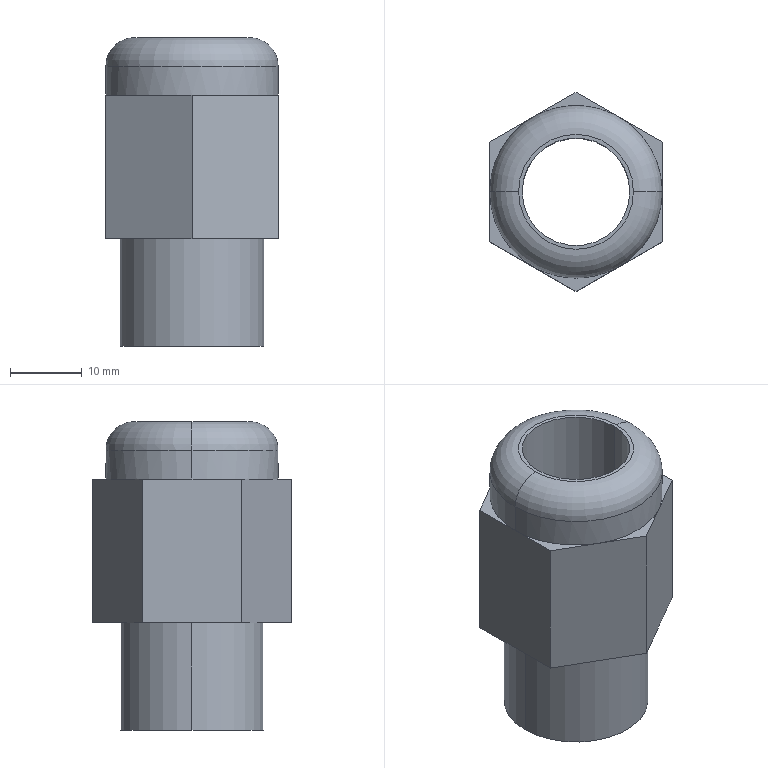Part | SolidWorks | features ICE 2, Extrusion 1, Fillet 1 | 1 solid | 23 faces | box 24 x 27.713 x 43 mm | volume 10470 mm3 | plane 15 | cylinder 6 | torus 2 | commonest cylinder face diameters 15 x2 20 x2 24 x2
STEP:
#1=CARTESIAN_POINT('',(-10.,0.,-15.));
#2=VERTEX_POINT('',#1);
#3=CARTESIAN_POINT('',(10.,0.,-15.));
#4=VERTEX_POINT('',#3);
#5=CARTESIAN_POINT('',(0.,0.,-15.));
#6=DIRECTION('',(0.,0.,-1.));
#7=DIRECTION('',(-1.,0.,0.));
#8=AXIS2_PLACEMENT_3D('',#5,#6,#7);
#9=CIRCLE('',#8,10.);
#10=EDGE_CURVE('',#2,#4,#9,.T.);
#11=ORIENTED_EDGE('',*,*,#10,.F.);
#12=CARTESIAN_POINT('',(-10.,0.,0.));
#13=VERTEX_POINT('',#12);
#14=CARTESIAN_POINT('',(-10.,0.,-15.));
#15=DIRECTION('',(0.,0.,1.));
#16=VECTOR('',#15,1000.);
#17=LINE('',#14,#16);
#18=EDGE_CURVE('',#2,#13,#17,.T.);
#19=ORIENTED_EDGE('',*,*,#18,.T.);
#20=CARTESIAN_POINT('',(10.,0.,0.));
#21=VERTEX_POINT('',#20);
#22=CARTESIAN_POINT('',(0.,0.,0.));
#23=DIRECTION('',(0.,0.,-1.));
#24=DIRECTION('',(1.,0.,0.));
#25=AXIS2_PLACEMENT_3D('',#22,#23,#24);
#26=CIRCLE('',#25,10.);
#27=EDGE_CURVE('',#13,#21,#26,.T.);
#28=ORIENTED_EDGE('',*,*,#27,.T.);
#29=CARTESIAN_POINT('',(10.,0.,-15.));
#30=DIRECTION('',(0.,0.,1.));
#31=VECTOR('',#30,1000.);
#32=LINE('',#29,#31);
#33=EDGE_CURVE('',#4,#21,#32,.T.);
#34=ORIENTED_EDGE('',*,*,#33,.F.);
#35=EDGE_LOOP('',(#11,#19,#28,#34));
#36=FACE_OUTER_BOUND('',#35,.T.);
#37=CARTESIAN_POINT('',(0.,0.,-15.));
#38=DIRECTION('',(0.,0.,1.));
#39=DIRECTION('',(1.,0.,0.));
#40=AXIS2_PLACEMENT_3D('',#37,#38,#39);
#41=CYLINDRICAL_SURFACE('',#40,10.);
#42=ADVANCED_FACE('',(#36),#41,.T.);
#43=CARTESIAN_POINT('',(-12.,0.,24.));
#44=VERTEX_POINT('',#43);
#45=CARTESIAN_POINT('',(12.,0.,24.));
#46=VERTEX_POINT('',#45);
#47=CARTESIAN_POINT('',(0.,0.,24.));
#48=DIRECTION('',(0.,0.,-1.));
#49=DIRECTION('',(1.,0.,0.));
#50=AXIS2_PLACEMENT_3D('',#47,#48,#49);
#51=CIRCLE('',#50,12.);
#52=EDGE_CURVE('',#44,#46,#51,.T.);
#53=ORIENTED_EDGE('',*,*,#52,.F.);
#54=CARTESIAN_POINT('',(-8.,0.,28.));
#55=VERTEX_POINT('',#54);
#56=CARTESIAN_POINT('',(-8.,0.,24.));
#57=DIRECTION('',(0.,1.,0.));
#58=DIRECTION('',(-1.,0.,0.));
#59=AXIS2_PLACEMENT_3D('',#56,#57,#58);
#60=CIRCLE('',#59,4.);
#61=EDGE_CURVE('',#44,#55,#60,.T.);
#62=ORIENTED_EDGE('',*,*,#61,.T.);
#63=CARTESIAN_POINT('',(8.,0.,28.));
#64=VERTEX_POINT('',#63);
#65=CARTESIAN_POINT('',(0.,0.,28.));
#66=DIRECTION('',(0.,0.,1.));
#67=DIRECTION('',(1.,0.,0.));
#68=AXIS2_PLACEMENT_3D('',#65,#66,#67);
#69=CIRCLE('',#68,8.);
#70=EDGE_CURVE('',#64,#55,#69,.T.);
#71=ORIENTED_EDGE('',*,*,#70,.F.);
#72=CARTESIAN_POINT('',(8.,0.,24.));
#73=DIRECTION('',(0.,-1.,0.));
#74=DIRECTION('',(0.,0.,-1.));
#75=AXIS2_PLACEMENT_3D('',#72,#73,#74);
#76=CIRCLE('',#75,4.);
#77=EDGE_CURVE('',#46,#64,#76,.T.);
#78=ORIENTED_EDGE('',*,*,#77,.F.);
#79=EDGE_LOOP('',(#53,#62,#71,#78));
#80=FACE_OUTER_BOUND('',#79,.T.);
#81=CARTESIAN_POINT('',(0.,0.,24.));
#82=DIRECTION('',(0.,0.,1.));
#83=DIRECTION('',(1.,0.,0.));
#84=AXIS2_PLACEMENT_3D('',#81,#82,#83);
#85=TOROIDAL_SURFACE('',#84,8.,4.);
#86=ADVANCED_FACE('',(#80),#85,.T.);
#87=ORIENTED_EDGE('',*,*,#52,.T.);
#88=CARTESIAN_POINT('',(12.,0.,20.));
#89=VERTEX_POINT('',#88);
#90=CARTESIAN_POINT('',(12.,0.,28.));
#91=DIRECTION('',(0.,0.,-1.));
#92=VECTOR('',#91,1000.);
#93=LINE('',#90,#92);
#94=EDGE_CURVE('',#46,#89,#93,.T.);
#95=ORIENTED_EDGE('',*,*,#94,.T.);
#96=CARTESIAN_POINT('',(6.,10.392,20.));
#97=VERTEX_POINT('',#96);
#98=CARTESIAN_POINT('',(0.,0.,20.));
#99=DIRECTION('',(0.,0.,1.));
#100=DIRECTION('',(1.,0.,0.));
#101=AXIS2_PLACEMENT_3D('',#98,#99,#100);
#102=CIRCLE('',#101,12.);
#103=EDGE_CURVE('',#89,#97,#102,.T.);
#104=ORIENTED_EDGE('',*,*,#103,.T.);
#105=CARTESIAN_POINT('',(-6.,10.392,20.));
#106=VERTEX_POINT('',#105);
#107=CARTESIAN_POINT('',(0.,0.,20.));
#108=DIRECTION('',(0.,0.,1.));
#109=DIRECTION('',(1.,0.,0.));
#110=AXIS2_PLACEMENT_3D('',#107,#108,#109);
#111=CIRCLE('',#110,12.);
#112=EDGE_CURVE('',#97,#106,#111,.T.);
#113=ORIENTED_EDGE('',*,*,#112,.T.);
#114=CARTESIAN_POINT('',(-12.,0.,20.));
#115=VERTEX_POINT('',#114);
#116=CARTESIAN_POINT('',(0.,0.,20.));
#117=DIRECTION('',(0.,0.,1.));
#118=DIRECTION('',(1.,0.,0.));
#119=AXIS2_PLACEMENT_3D('',#116,#117,#118);
#120=CIRCLE('',#119,12.);
#121=EDGE_CURVE('',#106,#115,#120,.T.);
#122=ORIENTED_EDGE('',*,*,#121,.T.);
#123=CARTESIAN_POINT('',(-12.,0.,28.));
#124=DIRECTION('',(0.,0.,-1.));
#125=VECTOR('',#124,1000.);
#126=LINE('',#123,#125);
#127=EDGE_CURVE('',#44,#115,#126,.T.);
#128=ORIENTED_EDGE('',*,*,#127,.F.);
#129=EDGE_LOOP('',(#87,#95,#104,#113,#122,#128));
#130=FACE_OUTER_BOUND('',#129,.T.);
#131=CARTESIAN_POINT('',(0.,0.,28.));
#132=DIRECTION('',(0.,0.,-1.));
#133=DIRECTION('',(-1.,0.,0.));
#134=AXIS2_PLACEMENT_3D('',#131,#132,#133);
#135=CYLINDRICAL_SURFACE('',#134,12.);
#136=ADVANCED_FACE('',(#130),#135,.T.);
#137=CARTESIAN_POINT('',(-7.5,0.,28.));
#138=VERTEX_POINT('',#137);
#139=CARTESIAN_POINT('',(7.5,0.,28.));
#140=VERTEX_POINT('',#139);
#141=CARTESIAN_POINT('',(0.,0.,28.));
#142=DIRECTION('',(0.,0.,1.));
#143=DIRECTION('',(1.,0.,0.));
#144=AXIS2_PLACEMENT_3D('',#141,#142,#143);
#145=CIRCLE('',#144,7.5);
#146=EDGE_CURVE('',#138,#140,#145,.T.);
#147=ORIENTED_EDGE('',*,*,#146,.T.);
#148=CARTESIAN_POINT('',(7.5,0.,-15.));
#149=VERTEX_POINT('',#148);
#150=CARTESIAN_POINT('',(7.5,0.,20.));
#151=DIRECTION('',(0.,0.,-1.));
#152=VECTOR('',#151,1000.);
#153=LINE('',#150,#152);
#154=EDGE_CURVE('',#140,#149,#153,.T.);
#155=ORIENTED_EDGE('',*,*,#154,.T.);
#156=CARTESIAN_POINT('',(-7.5,0.,-15.));
#157=VERTEX_POINT('',#156);
#158=CARTESIAN_POINT('',(0.,0.,-15.));
#159=DIRECTION('',(0.,0.,-1.));
#160=DIRECTION('',(-1.,0.,0.));
#161=AXIS2_PLACEMENT_3D('',#158,#159,#160);
#162=CIRCLE('',#161,7.5);
#163=EDGE_CURVE('',#149,#157,#162,.T.);
#164=ORIENTED_EDGE('',*,*,#163,.T.);
#165=CARTESIAN_POINT('',(-7.5,0.,20.));
#166=DIRECTION('',(0.,0.,-1.));
#167=VECTOR('',#166,1000.);
#168=LINE('',#165,#167);
#169=EDGE_CURVE('',#138,#157,#168,.T.);
#170=ORIENTED_EDGE('',*,*,#169,.F.);
#171=EDGE_LOOP('',(#147,#155,#164,#170));
#172=FACE_OUTER_BOUND('',#171,.T.);
#173=CARTESIAN_POINT('',(0.,0.,20.));
#174=DIRECTION('',(0.,0.,-1.));
#175=DIRECTION('',(-1.,0.,0.));
#176=AXIS2_PLACEMENT_3D('',#173,#174,#175);
#177=CYLINDRICAL_SURFACE('',#176,7.5);
#178=ADVANCED_FACE('',(#172),#177,.F.);
#179=CARTESIAN_POINT('',(12.,6.928,0.));
#180=VERTEX_POINT('',#179);
#181=CARTESIAN_POINT('',(0.,13.856,0.));
#182=VERTEX_POINT('',#181);
#183=CARTESIAN_POINT('',(12.,6.928,0.));
#184=DIRECTION('',(-0.866,0.5,0.));
#185=VECTOR('',#184,1000.);
#186=LINE('',#183,#185);
#187=EDGE_CURVE('',#180,#182,#186,.T.);
#188=ORIENTED_EDGE('',*,*,#187,.F.);
#189=CARTESIAN_POINT('',(12.,-6.928,0.));
#190=VERTEX_POINT('',#189);
#191=CARTESIAN_POINT('',(12.,-6.928,0.));
#192=DIRECTION('',(0.,1.,0.));
#193=VECTOR('',#192,1000.);
#194=LINE('',#191,#193);
#195=EDGE_CURVE('',#190,#180,#194,.T.);
#196=ORIENTED_EDGE('',*,*,#195,.F.);
#197=CARTESIAN_POINT('',(0.,-13.856,0.));
#198=VERTEX_POINT('',#197);
#199=CARTESIAN_POINT('',(0.,-13.856,0.));
#200=DIRECTION('',(0.866,0.5,0.));
#201=VECTOR('',#200,1000.);
#202=LINE('',#199,#201);
#203=EDGE_CURVE('',#198,#190,#202,.T.);
#204=ORIENTED_EDGE('',*,*,#203,.F.);
#205=CARTESIAN_POINT('',(-12.,-6.928,0.));
#206=VERTEX_POINT('',#205);
#207=CARTESIAN_POINT('',(-12.,-6.928,0.));
#208=DIRECTION('',(0.866,-0.5,0.));
#209=VECTOR('',#208,1000.);
#210=LINE('',#207,#209);
#211=EDGE_CURVE('',#206,#198,#210,.T.);
#212=ORIENTED_EDGE('',*,*,#211,.F.);
#213=CARTESIAN_POINT('',(-12.,6.928,0.));
#214=VERTEX_POINT('',#213);
#215=CARTESIAN_POINT('',(-12.,6.928,0.));
#216=DIRECTION('',(0.,-1.,0.));
#217=VECTOR('',#216,1000.);
#218=LINE('',#215,#217);
#219=EDGE_CURVE('',#214,#206,#218,.T.);
#220=ORIENTED_EDGE('',*,*,#219,.F.);
#221=CARTESIAN_POINT('',(0.,13.856,0.));
#222=DIRECTION('',(-0.866,-0.5,0.));
#223=VECTOR('',#222,1000.);
#224=LINE('',#221,#223);
#225=EDGE_CURVE('',#182,#214,#224,.T.);
#226=ORIENTED_EDGE('',*,*,#225,.F.);
#227=EDGE_LOOP('',(#188,#196,#204,#212,#220,#226));
#228=FACE_OUTER_BOUND('',#227,.T.);
#229=CARTESIAN_POINT('',(0.,0.,0.));
#230=DIRECTION('',(0.,0.,-1.));
#231=DIRECTION('',(1.,0.,0.));
#232=AXIS2_PLACEMENT_3D('',#229,#230,#231);
#233=CIRCLE('',#232,10.);
#234=EDGE_CURVE('',#21,#13,#233,.T.);
#235=ORIENTED_EDGE('',*,*,#234,.F.);
#236=ORIENTED_EDGE('',*,*,#27,.F.);
#237=EDGE_LOOP('',(#235,#236));
#238=FACE_BOUND('',#237,.T.);
#239=CARTESIAN_POINT('',(0.,0.,0.));
#240=DIRECTION('',(0.,0.,1.));
#241=DIRECTION('',(1.,0.,0.));
#242=AXIS2_PLACEMENT_3D('',#239,#240,#241);
#243=PLANE('',#242);
#244=ADVANCED_FACE('',(#228,#238),#243,.F.);
#245=ORIENTED_EDGE('',*,*,#103,.F.);
#246=CARTESIAN_POINT('',(12.,6.928,20.));
#247=VERTEX_POINT('',#246);
#248=CARTESIAN_POINT('',(12.,-6.928,20.));
#249=DIRECTION('',(0.,1.,0.));
#250=VECTOR('',#249,1000.);
#251=LINE('',#248,#250);
#252=EDGE_CURVE('',#89,#247,#251,.T.);
#253=ORIENTED_EDGE('',*,*,#252,.T.);
#254=CARTESIAN_POINT('',(12.,6.928,20.));
#255=DIRECTION('',(-0.866,0.5,0.));
#256=VECTOR('',#255,1000.);
#257=LINE('',#254,#256);
#258=EDGE_CURVE('',#247,#97,#257,.T.);
#259=ORIENTED_EDGE('',*,*,#258,.T.);
#260=EDGE_LOOP('',(#245,#253,#259));
#261=FACE_OUTER_BOUND('',#260,.T.);
#262=CARTESIAN_POINT('',(0.,0.,20.));
#263=DIRECTION('',(0.,0.,1.));
#264=DIRECTION('',(1.,0.,0.));
#265=AXIS2_PLACEMENT_3D('',#262,#263,#264);
#266=PLANE('',#265);
#267=ADVANCED_FACE('',(#261),#266,.T.);
#268=ORIENTED_EDGE('',*,*,#112,.F.);
#269=CARTESIAN_POINT('',(0.,13.856,20.));
#270=VERTEX_POINT('',#269);
#271=CARTESIAN_POINT('',(12.,6.928,20.));
#272=DIRECTION('',(-0.866,0.5,0.));
#273=VECTOR('',#272,1000.);
#274=LINE('',#271,#273);
#275=EDGE_CURVE('',#97,#270,#274,.T.);
#276=ORIENTED_EDGE('',*,*,#275,.T.);
#277=CARTESIAN_POINT('',(0.,13.856,20.));
#278=DIRECTION('',(-0.866,-0.5,0.));
#279=VECTOR('',#278,1000.);
#280=LINE('',#277,#279);
#281=EDGE_CURVE('',#270,#106,#280,.T.);
#282=ORIENTED_EDGE('',*,*,#281,.T.);
#283=EDGE_LOOP('',(#268,#276,#282));
#284=FACE_OUTER_BOUND('',#283,.T.);
#285=CARTESIAN_POINT('',(0.,0.,20.));
#286=DIRECTION('',(0.,0.,1.));
#287=DIRECTION('',(1.,0.,0.));
#288=AXIS2_PLACEMENT_3D('',#285,#286,#287);
#289=PLANE('',#288);
#290=ADVANCED_FACE('',(#284),#289,.T.);
#291=ORIENTED_EDGE('',*,*,#121,.F.);
#292=CARTESIAN_POINT('',(-12.,6.928,20.));
#293=VERTEX_POINT('',#292);
#294=CARTESIAN_POINT('',(0.,13.856,20.));
#295=DIRECTION('',(-0.866,-0.5,0.));
#296=VECTOR('',#295,1000.);
#297=LINE('',#294,#296);
#298=EDGE_CURVE('',#106,#293,#297,.T.);
#299=ORIENTED_EDGE('',*,*,#298,.T.);
#300=CARTESIAN_POINT('',(-12.,6.928,20.));
#301=DIRECTION('',(0.,-1.,0.));
#302=VECTOR('',#301,1000.);
#303=LINE('',#300,#302);
#304=EDGE_CURVE('',#293,#115,#303,.T.);
#305=ORIENTED_EDGE('',*,*,#304,.T.);
#306=EDGE_LOOP('',(#291,#299,#305));
#307=FACE_OUTER_BOUND('',#306,.T.);
#308=CARTESIAN_POINT('',(0.,0.,20.));
#309=DIRECTION('',(0.,0.,1.));
#310=DIRECTION('',(1.,0.,0.));
#311=AXIS2_PLACEMENT_3D('',#308,#309,#310);
#312=PLANE('',#311);
#313=ADVANCED_FACE('',(#307),#312,.T.);
#314=CARTESIAN_POINT('',(-6.,-10.392,20.));
#315=VERTEX_POINT('',#314);
#316=CARTESIAN_POINT('',(0.,0.,20.));
#317=DIRECTION('',(0.,0.,1.));
#318=DIRECTION('',(1.,0.,0.));
#319=AXIS2_PLACEMENT_3D('',#316,#317,#318);
#320=CIRCLE('',#319,12.);
#321=EDGE_CURVE('',#115,#315,#320,.T.);
#322=ORIENTED_EDGE('',*,*,#321,.F.);
#323=CARTESIAN_POINT('',(-12.,-6.928,20.));
#324=VERTEX_POINT('',#323);
#325=CARTESIAN_POINT('',(-12.,6.928,20.));
#326=DIRECTION('',(0.,-1.,0.));
#327=VECTOR('',#326,1000.);
#328=LINE('',#325,#327);
#329=EDGE_CURVE('',#115,#324,#328,.T.);
#330=ORIENTED_EDGE('',*,*,#329,.T.);
#331=CARTESIAN_POINT('',(-12.,-6.928,20.));
#332=DIRECTION('',(0.866,-0.5,0.));
#333=VECTOR('',#332,1000.);
#334=LINE('',#331,#333);
#335=EDGE_CURVE('',#324,#315,#334,.T.);
#336=ORIENTED_EDGE('',*,*,#335,.T.);
#337=EDGE_LOOP('',(#322,#330,#336));
#338=FACE_OUTER_BOUND('',#337,.T.);
#339=CARTESIAN_POINT('',(0.,0.,20.));
#340=DIRECTION('',(0.,0.,1.));
#341=DIRECTION('',(1.,0.,0.));
#342=AXIS2_PLACEMENT_3D('',#339,#340,#341);
#343=PLANE('',#342);
#344=ADVANCED_FACE('',(#338),#343,.T.);
#345=CARTESIAN_POINT('',(6.,-10.392,20.));
#346=VERTEX_POINT('',#345);
#347=CARTESIAN_POINT('',(0.,0.,20.));
#348=DIRECTION('',(0.,0.,1.));
#349=DIRECTION('',(1.,0.,0.));
#350=AXIS2_PLACEMENT_3D('',#347,#348,#349);
#351=CIRCLE('',#350,12.);
#352=EDGE_CURVE('',#315,#346,#351,.T.);
#353=ORIENTED_EDGE('',*,*,#352,.F.);
#354=CARTESIAN_POINT('',(0.,-13.856,20.));
#355=VERTEX_POINT('',#354);
#356=CARTESIAN_POINT('',(-12.,-6.928,20.));
#357=DIRECTION('',(0.866,-0.5,0.));
#358=VECTOR('',#357,1000.);
#359=LINE('',#356,#358);
#360=EDGE_CURVE('',#315,#355,#359,.T.);
#361=ORIENTED_EDGE('',*,*,#360,.T.);
#362=CARTESIAN_POINT('',(0.,-13.856,20.));
#363=DIRECTION('',(0.866,0.5,0.));
#364=VECTOR('',#363,1000.);
#365=LINE('',#362,#364);
#366=EDGE_CURVE('',#355,#346,#365,.T.);
#367=ORIENTED_EDGE('',*,*,#366,.T.);
#368=EDGE_LOOP('',(#353,#361,#367));
#369=FACE_OUTER_BOUND('',#368,.T.);
#370=CARTESIAN_POINT('',(0.,0.,20.));
#371=DIRECTION('',(0.,0.,1.));
#372=DIRECTION('',(1.,0.,0.));
#373=AXIS2_PLACEMENT_3D('',#370,#371,#372);
#374=PLANE('',#373);
#375=ADVANCED_FACE('',(#369),#374,.T.);
#376=CARTESIAN_POINT('',(0.,0.,20.));
#377=DIRECTION('',(0.,0.,1.));
#378=DIRECTION('',(1.,0.,0.));
#379=AXIS2_PLACEMENT_3D('',#376,#377,#378);
#380=CIRCLE('',#379,12.);
#381=EDGE_CURVE('',#346,#89,#380,.T.);
#382=ORIENTED_EDGE('',*,*,#381,.F.);
#383=CARTESIAN_POINT('',(12.,-6.928,20.));
#384=VERTEX_POINT('',#383);
#385=CARTESIAN_POINT('',(0.,-13.856,20.));
#386=DIRECTION('',(0.866,0.5,0.));
#387=VECTOR('',#386,1000.);
#388=LINE('',#385,#387);
#389=EDGE_CURVE('',#346,#384,#388,.T.);
#390=ORIENTED_EDGE('',*,*,#389,.T.);
#391=CARTESIAN_POINT('',(12.,-6.928,20.));
#392=DIRECTION('',(0.,1.,0.));
#393=VECTOR('',#392,1000.);
#394=LINE('',#391,#393);
#395=EDGE_CURVE('',#384,#89,#394,.T.);
#396=ORIENTED_EDGE('',*,*,#395,.T.);
#397=EDGE_LOOP('',(#382,#390,#396));
#398=FACE_OUTER_BOUND('',#397,.T.);
#399=CARTESIAN_POINT('',(0.,0.,20.));
#400=DIRECTION('',(0.,0.,1.));
#401=DIRECTION('',(1.,0.,0.));
#402=AXIS2_PLACEMENT_3D('',#399,#400,#401);
#403=PLANE('',#402);
#404=ADVANCED_FACE('',(#398),#403,.T.);
#405=ORIENTED_EDGE('',*,*,#187,.T.);
#406=CARTESIAN_POINT('',(0.,13.856,20.));
#407=DIRECTION('',(0.,0.,-1.));
#408=VECTOR('',#407,1000.);
#409=LINE('',#406,#408);
#410=EDGE_CURVE('',#270,#182,#409,.T.);
#411=ORIENTED_EDGE('',*,*,#410,.F.);
#412=ORIENTED_EDGE('',*,*,#275,.F.);
#413=ORIENTED_EDGE('',*,*,#258,.F.);
#414=CARTESIAN_POINT('',(12.,6.928,20.));
#415=DIRECTION('',(0.,0.,-1.));
#416=VECTOR('',#415,1000.);
#417=LINE('',#414,#416);
#418=EDGE_CURVE('',#247,#180,#417,.T.);
#419=ORIENTED_EDGE('',*,*,#418,.T.);
#420=EDGE_LOOP('',(#405,#411,#412,#413,#419));
#421=FACE_OUTER_BOUND('',#420,.T.);
#422=CARTESIAN_POINT('',(12.,6.928,20.));
#423=DIRECTION('',(-0.5,-0.866,0.));
#424=DIRECTION('',(0.866,-0.5,0.));
#425=AXIS2_PLACEMENT_3D('',#422,#423,#424);
#426=PLANE('',#425);
#427=ADVANCED_FACE('',(#421),#426,.F.);
#428=ORIENTED_EDGE('',*,*,#225,.T.);
#429=CARTESIAN_POINT('',(-12.,6.928,20.));
#430=DIRECTION('',(0.,0.,-1.));
#431=VECTOR('',#430,1000.);
#432=LINE('',#429,#431);
#433=EDGE_CURVE('',#293,#214,#432,.T.);
#434=ORIENTED_EDGE('',*,*,#433,.F.);
#435=ORIENTED_EDGE('',*,*,#298,.F.);
#436=ORIENTED_EDGE('',*,*,#281,.F.);
#437=ORIENTED_EDGE('',*,*,#410,.T.);
#438=EDGE_LOOP('',(#428,#434,#435,#436,#437));
#439=FACE_OUTER_BOUND('',#438,.T.);
#440=CARTESIAN_POINT('',(0.,13.856,20.));
#441=DIRECTION('',(0.5,-0.866,0.));
#442=DIRECTION('',(0.866,0.5,0.));
#443=AXIS2_PLACEMENT_3D('',#440,#441,#442);
#444=PLANE('',#443);
#445=ADVANCED_FACE('',(#439),#444,.F.);
#446=ORIENTED_EDGE('',*,*,#219,.T.);
#447=CARTESIAN_POINT('',(-12.,-6.928,20.));
#448=DIRECTION('',(0.,0.,-1.));
#449=VECTOR('',#448,1000.);
#450=LINE('',#447,#449);
#451=EDGE_CURVE('',#324,#206,#450,.T.);
#452=ORIENTED_EDGE('',*,*,#451,.F.);
#453=ORIENTED_EDGE('',*,*,#329,.F.);
#454=ORIENTED_EDGE('',*,*,#304,.F.);
#455=ORIENTED_EDGE('',*,*,#433,.T.);
#456=EDGE_LOOP('',(#446,#452,#453,#454,#455));
#457=FACE_OUTER_BOUND('',#456,.T.);
#458=CARTESIAN_POINT('',(-12.,6.928,20.));
#459=DIRECTION('',(1.,0.,0.));
#460=DIRECTION('',(0.,1.,0.));
#461=AXIS2_PLACEMENT_3D('',#458,#459,#460);
#462=PLANE('',#461);
#463=ADVANCED_FACE('',(#457),#462,.F.);
#464=ORIENTED_EDGE('',*,*,#211,.T.);
#465=CARTESIAN_POINT('',(0.,-13.856,20.));
#466=DIRECTION('',(0.,0.,-1.));
#467=VECTOR('',#466,1000.);
#468=LINE('',#465,#467);
#469=EDGE_CURVE('',#355,#198,#468,.T.);
#470=ORIENTED_EDGE('',*,*,#469,.F.);
#471=ORIENTED_EDGE('',*,*,#360,.F.);
#472=ORIENTED_EDGE('',*,*,#335,.F.);
#473=ORIENTED_EDGE('',*,*,#451,.T.);
#474=EDGE_LOOP('',(#464,#470,#471,#472,#473));
#475=FACE_OUTER_BOUND('',#474,.T.);
#476=CARTESIAN_POINT('',(-12.,-6.928,20.));
#477=DIRECTION('',(0.5,0.866,0.));
#478=DIRECTION('',(-0.866,0.5,0.));
#479=AXIS2_PLACEMENT_3D('',#476,#477,#478);
#480=PLANE('',#479);
#481=ADVANCED_FACE('',(#475),#480,.F.);
#482=ORIENTED_EDGE('',*,*,#203,.T.);
#483=CARTESIAN_POINT('',(12.,-6.928,20.));
#484=DIRECTION('',(0.,0.,-1.));
#485=VECTOR('',#484,1000.);
#486=LINE('',#483,#485);
#487=EDGE_CURVE('',#384,#190,#486,.T.);
#488=ORIENTED_EDGE('',*,*,#487,.F.);
#489=ORIENTED_EDGE('',*,*,#389,.F.);
#490=ORIENTED_EDGE('',*,*,#366,.F.);
#491=ORIENTED_EDGE('',*,*,#469,.T.);
#492=EDGE_LOOP('',(#482,#488,#489,#490,#491));
#493=FACE_OUTER_BOUND('',#492,.T.);
#494=CARTESIAN_POINT('',(0.,-13.856,20.));
#495=DIRECTION('',(-0.5,0.866,0.));
#496=DIRECTION('',(-0.866,-0.5,0.));
#497=AXIS2_PLACEMENT_3D('',#494,#495,#496);
#498=PLANE('',#497);
#499=ADVANCED_FACE('',(#493),#498,.F.);
#500=ORIENTED_EDGE('',*,*,#195,.T.);
#501=ORIENTED_EDGE('',*,*,#418,.F.);
#502=ORIENTED_EDGE('',*,*,#252,.F.);
#503=ORIENTED_EDGE('',*,*,#395,.F.);
#504=ORIENTED_EDGE('',*,*,#487,.T.);
#505=EDGE_LOOP('',(#500,#501,#502,#503,#504));
#506=FACE_OUTER_BOUND('',#505,.T.);
#507=CARTESIAN_POINT('',(12.,-6.928,20.));
#508=DIRECTION('',(-1.,0.,0.));
#509=DIRECTION('',(0.,-1.,0.));
#510=AXIS2_PLACEMENT_3D('',#507,#508,#509);
#511=PLANE('',#510);
#512=ADVANCED_FACE('',(#506),#511,.F.);
#513=ORIENTED_EDGE('',*,*,#154,.F.);
#514=CARTESIAN_POINT('',(0.,0.,28.));
#515=DIRECTION('',(0.,0.,1.));
#516=DIRECTION('',(1.,0.,0.));
#517=AXIS2_PLACEMENT_3D('',#514,#515,#516);
#518=CIRCLE('',#517,7.5);
#519=EDGE_CURVE('',#140,#138,#518,.T.);
#520=ORIENTED_EDGE('',*,*,#519,.T.);
#521=ORIENTED_EDGE('',*,*,#169,.T.);
#522=CARTESIAN_POINT('',(0.,0.,-15.));
#523=DIRECTION('',(0.,0.,-1.));
#524=DIRECTION('',(-1.,0.,0.));
#525=AXIS2_PLACEMENT_3D('',#522,#523,#524);
#526=CIRCLE('',#525,7.5);
#527=EDGE_CURVE('',#157,#149,#526,.T.);
#528=ORIENTED_EDGE('',*,*,#527,.T.);
#529=EDGE_LOOP('',(#513,#520,#521,#528));
#530=FACE_OUTER_BOUND('',#529,.T.);
#531=CARTESIAN_POINT('',(0.,0.,20.));
#532=DIRECTION('',(0.,0.,-1.));
#533=DIRECTION('',(-1.,0.,0.));
#534=AXIS2_PLACEMENT_3D('',#531,#532,#533);
#535=CYLINDRICAL_SURFACE('',#534,7.5);
#536=ADVANCED_FACE('',(#530),#535,.F.);
#537=ORIENTED_EDGE('',*,*,#70,.T.);
#538=CARTESIAN_POINT('',(0.,0.,28.));
#539=DIRECTION('',(0.,0.,1.));
#540=DIRECTION('',(1.,0.,0.));
#541=AXIS2_PLACEMENT_3D('',#538,#539,#540);
#542=CIRCLE('',#541,8.);
#543=EDGE_CURVE('',#55,#64,#542,.T.);
#544=ORIENTED_EDGE('',*,*,#543,.T.);
#545=EDGE_LOOP('',(#537,#544));
#546=FACE_OUTER_BOUND('',#545,.T.);
#547=ORIENTED_EDGE('',*,*,#146,.F.);
#548=ORIENTED_EDGE('',*,*,#519,.F.);
#549=EDGE_LOOP('',(#547,#548));
#550=FACE_BOUND('',#549,.T.);
#551=CARTESIAN_POINT('',(0.,0.,28.));
#552=DIRECTION('',(0.,0.,1.));
#553=DIRECTION('',(1.,0.,0.));
#554=AXIS2_PLACEMENT_3D('',#551,#552,#553);
#555=PLANE('',#554);
#556=ADVANCED_FACE('',(#546,#550),#555,.T.);
#557=ORIENTED_EDGE('',*,*,#94,.F.);
#558=CARTESIAN_POINT('',(0.,0.,24.));
#559=DIRECTION('',(0.,0.,-1.));
#560=DIRECTION('',(1.,0.,0.));
#561=AXIS2_PLACEMENT_3D('',#558,#559,#560);
#562=CIRCLE('',#561,12.);
#563=EDGE_CURVE('',#46,#44,#562,.T.);
#564=ORIENTED_EDGE('',*,*,#563,.T.);
#565=ORIENTED_EDGE('',*,*,#127,.T.);
#566=ORIENTED_EDGE('',*,*,#321,.T.);
#567=ORIENTED_EDGE('',*,*,#352,.T.);
#568=ORIENTED_EDGE('',*,*,#381,.T.);
#569=EDGE_LOOP('',(#557,#564,#565,#566,#567,#568));
#570=FACE_OUTER_BOUND('',#569,.T.);
#571=CARTESIAN_POINT('',(0.,0.,28.));
#572=DIRECTION('',(0.,0.,-1.));
#573=DIRECTION('',(-1.,0.,0.));
#574=AXIS2_PLACEMENT_3D('',#571,#572,#573);
#575=CYLINDRICAL_SURFACE('',#574,12.);
#576=ADVANCED_FACE('',(#570),#575,.T.);
#577=ORIENTED_EDGE('',*,*,#61,.F.);
#578=ORIENTED_EDGE('',*,*,#563,.F.);
#579=ORIENTED_EDGE('',*,*,#77,.T.);
#580=ORIENTED_EDGE('',*,*,#543,.F.);
#581=EDGE_LOOP('',(#577,#578,#579,#580));
#582=FACE_OUTER_BOUND('',#581,.T.);
#583=CARTESIAN_POINT('',(0.,0.,24.));
#584=DIRECTION('',(0.,0.,1.));
#585=DIRECTION('',(1.,0.,0.));
#586=AXIS2_PLACEMENT_3D('',#583,#584,#585);
#587=TOROIDAL_SURFACE('',#586,8.,4.);
#588=ADVANCED_FACE('',(#582),#587,.T.);
#589=CARTESIAN_POINT('',(0.,0.,-15.));
#590=DIRECTION('',(0.,0.,-1.));
#591=DIRECTION('',(-1.,0.,0.));
#592=AXIS2_PLACEMENT_3D('',#589,#590,#591);
#593=CIRCLE('',#592,10.);
#594=EDGE_CURVE('',#4,#2,#593,.T.);
#595=ORIENTED_EDGE('',*,*,#594,.T.);
#596=ORIENTED_EDGE('',*,*,#10,.T.);
#597=EDGE_LOOP('',(#595,#596));
#598=FACE_OUTER_BOUND('',#597,.T.);
#599=ORIENTED_EDGE('',*,*,#527,.F.);
#600=ORIENTED_EDGE('',*,*,#163,.F.);
#601=EDGE_LOOP('',(#599,#600));
#602=FACE_BOUND('',#601,.T.);
#603=CARTESIAN_POINT('',(0.,0.,-15.));
#604=DIRECTION('',(0.,0.,-1.));
#605=DIRECTION('',(-1.,0.,0.));
#606=AXIS2_PLACEMENT_3D('',#603,#604,#605);
#607=PLANE('',#606);
#608=ADVANCED_FACE('',(#598,#602),#607,.T.);
#609=ORIENTED_EDGE('',*,*,#18,.F.);
#610=ORIENTED_EDGE('',*,*,#594,.F.);
#611=ORIENTED_EDGE('',*,*,#33,.T.);
#612=ORIENTED_EDGE('',*,*,#234,.T.);
#613=EDGE_LOOP('',(#609,#610,#611,#612));
#614=FACE_OUTER_BOUND('',#613,.T.);
#615=CARTESIAN_POINT('',(0.,0.,-15.));
#616=DIRECTION('',(0.,0.,1.));
#617=DIRECTION('',(1.,0.,0.));
#618=AXIS2_PLACEMENT_3D('',#615,#616,#617);
#619=CYLINDRICAL_SURFACE('',#618,10.);
#620=ADVANCED_FACE('',(#614),#619,.T.);
#621=CLOSED_SHELL('',(#42,#86,#136,#178,#244,#267,#290,#313,#344,#375,#404,#427,#445,#463,#481,#499,#512,#536,#556,#576,#588,#608,#620));
#622=MANIFOLD_SOLID_BREP('',#621);
#623=CARTESIAN_POINT('',(0.,0.,0.));
#624=DIRECTION('',(0.,0.,1.));
#625=DIRECTION('',(1.,0.,0.));
#626=AXIS2_PLACEMENT_3D('',#623,#624,#625);
#627=(LENGTH_UNIT()NAMED_UNIT(*)SI_UNIT(.MILLI.,.METRE.));
#628=UNCERTAINTY_MEASURE_WITH_UNIT(LENGTH_MEASURE(0.00001),#627,'','');
#629=(NAMED_UNIT(*)PLANE_ANGLE_UNIT()SI_UNIT($,.RADIAN.));
#630=(NAMED_UNIT(*)SI_UNIT($,.STERADIAN.)SOLID_ANGLE_UNIT());
#631=(GEOMETRIC_REPRESENTATION_CONTEXT(3)GLOBAL_UNCERTAINTY_ASSIGNED_CONTEXT((#628))GLOBAL_UNIT_ASSIGNED_CONTEXT((#627,#629,#630))REPRESENTATION_CONTEXT('',''));
#632=ADVANCED_BREP_SHAPE_REPRESENTATION('',(#622,#626),#631);